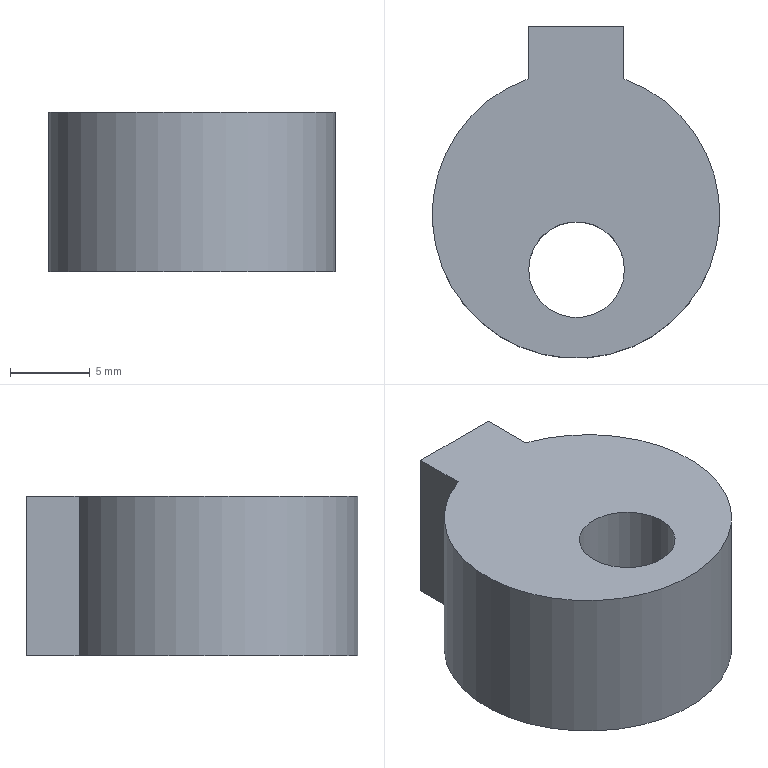NC program | NX | posted with a generic post | part box 18 x 20.8 x 10 mm
Lines 1 to 50 of 1937:
N10 G17 G21 G94 G90
(DRILLING , TOOL : 倒角D8-90度)
N12 T01 M6
N14 G53
N16 G17 G0 G90 X-3. Y7.085 S2000 M3
N18 G43 Z20. H1
N20 G94 G81 G99 Z-1.5 F200. R3.
N22 X3.
N24 X0.035 Y-4.853
N26 G80
N28 G0 X0.035 Y-4.853 Z20.
N30 M5
(DRILLING_COPY , TOOL : 钻头D4.0-54-83)
N32 T02 M6
N34 G53
N36 G17 G0 G90 X-3. Y7.085 S2000 M3
N38 G43 Z20. H2
N40 G94 G83 G99 Z-13. F200. Q2. R3.
N42 X3.
N44 G80
N46 G0 X3. Y7.085 Z20.
N48 M5
(DRILLING_COPY_1 , TOOL : 钻头D5.1-62-92)
N50 T03 M6
N52 G53
N54 G17 G0 G90 X0.035 Y-4.853 S2000 M3
N56 G43 Z20. H3
N58 G94 G83 G99 Z-20. F200. Q2. R3.
N60 G80
N62 G0 X0.035 Y-4.853 Z20.
N64 M5
(DRILLING_COPY_1_COPY , TOOL : 上排M6-23-D6-63)
N66 T04 M6
N68 G53
N70 G17 G0 G90 X0.035 Y-4.853 S300 M3
N72 G43 Z20. H4
N74 G84 G94 G99 Z-5. F300. R3.
N76 G80
N78 G0 X0.035 Y-4.853 Z20.
N80 M5